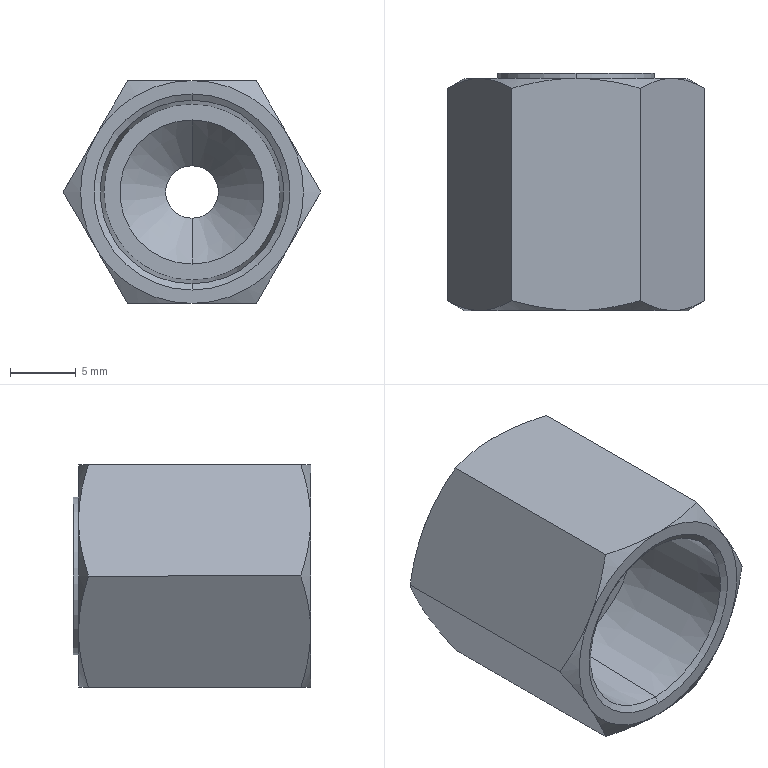Part | STEP file | AC40-04-KSTV-38JNR_AC3009A AF Drain-2 | 1 solid | 34 faces | box 19.63 x 18.1 x 17 mm | volume 2625 mm3 | cone 18 | plane 10 | cylinder 6 | commonest cylinder face diameters 4 x2 11 x2 12 x2